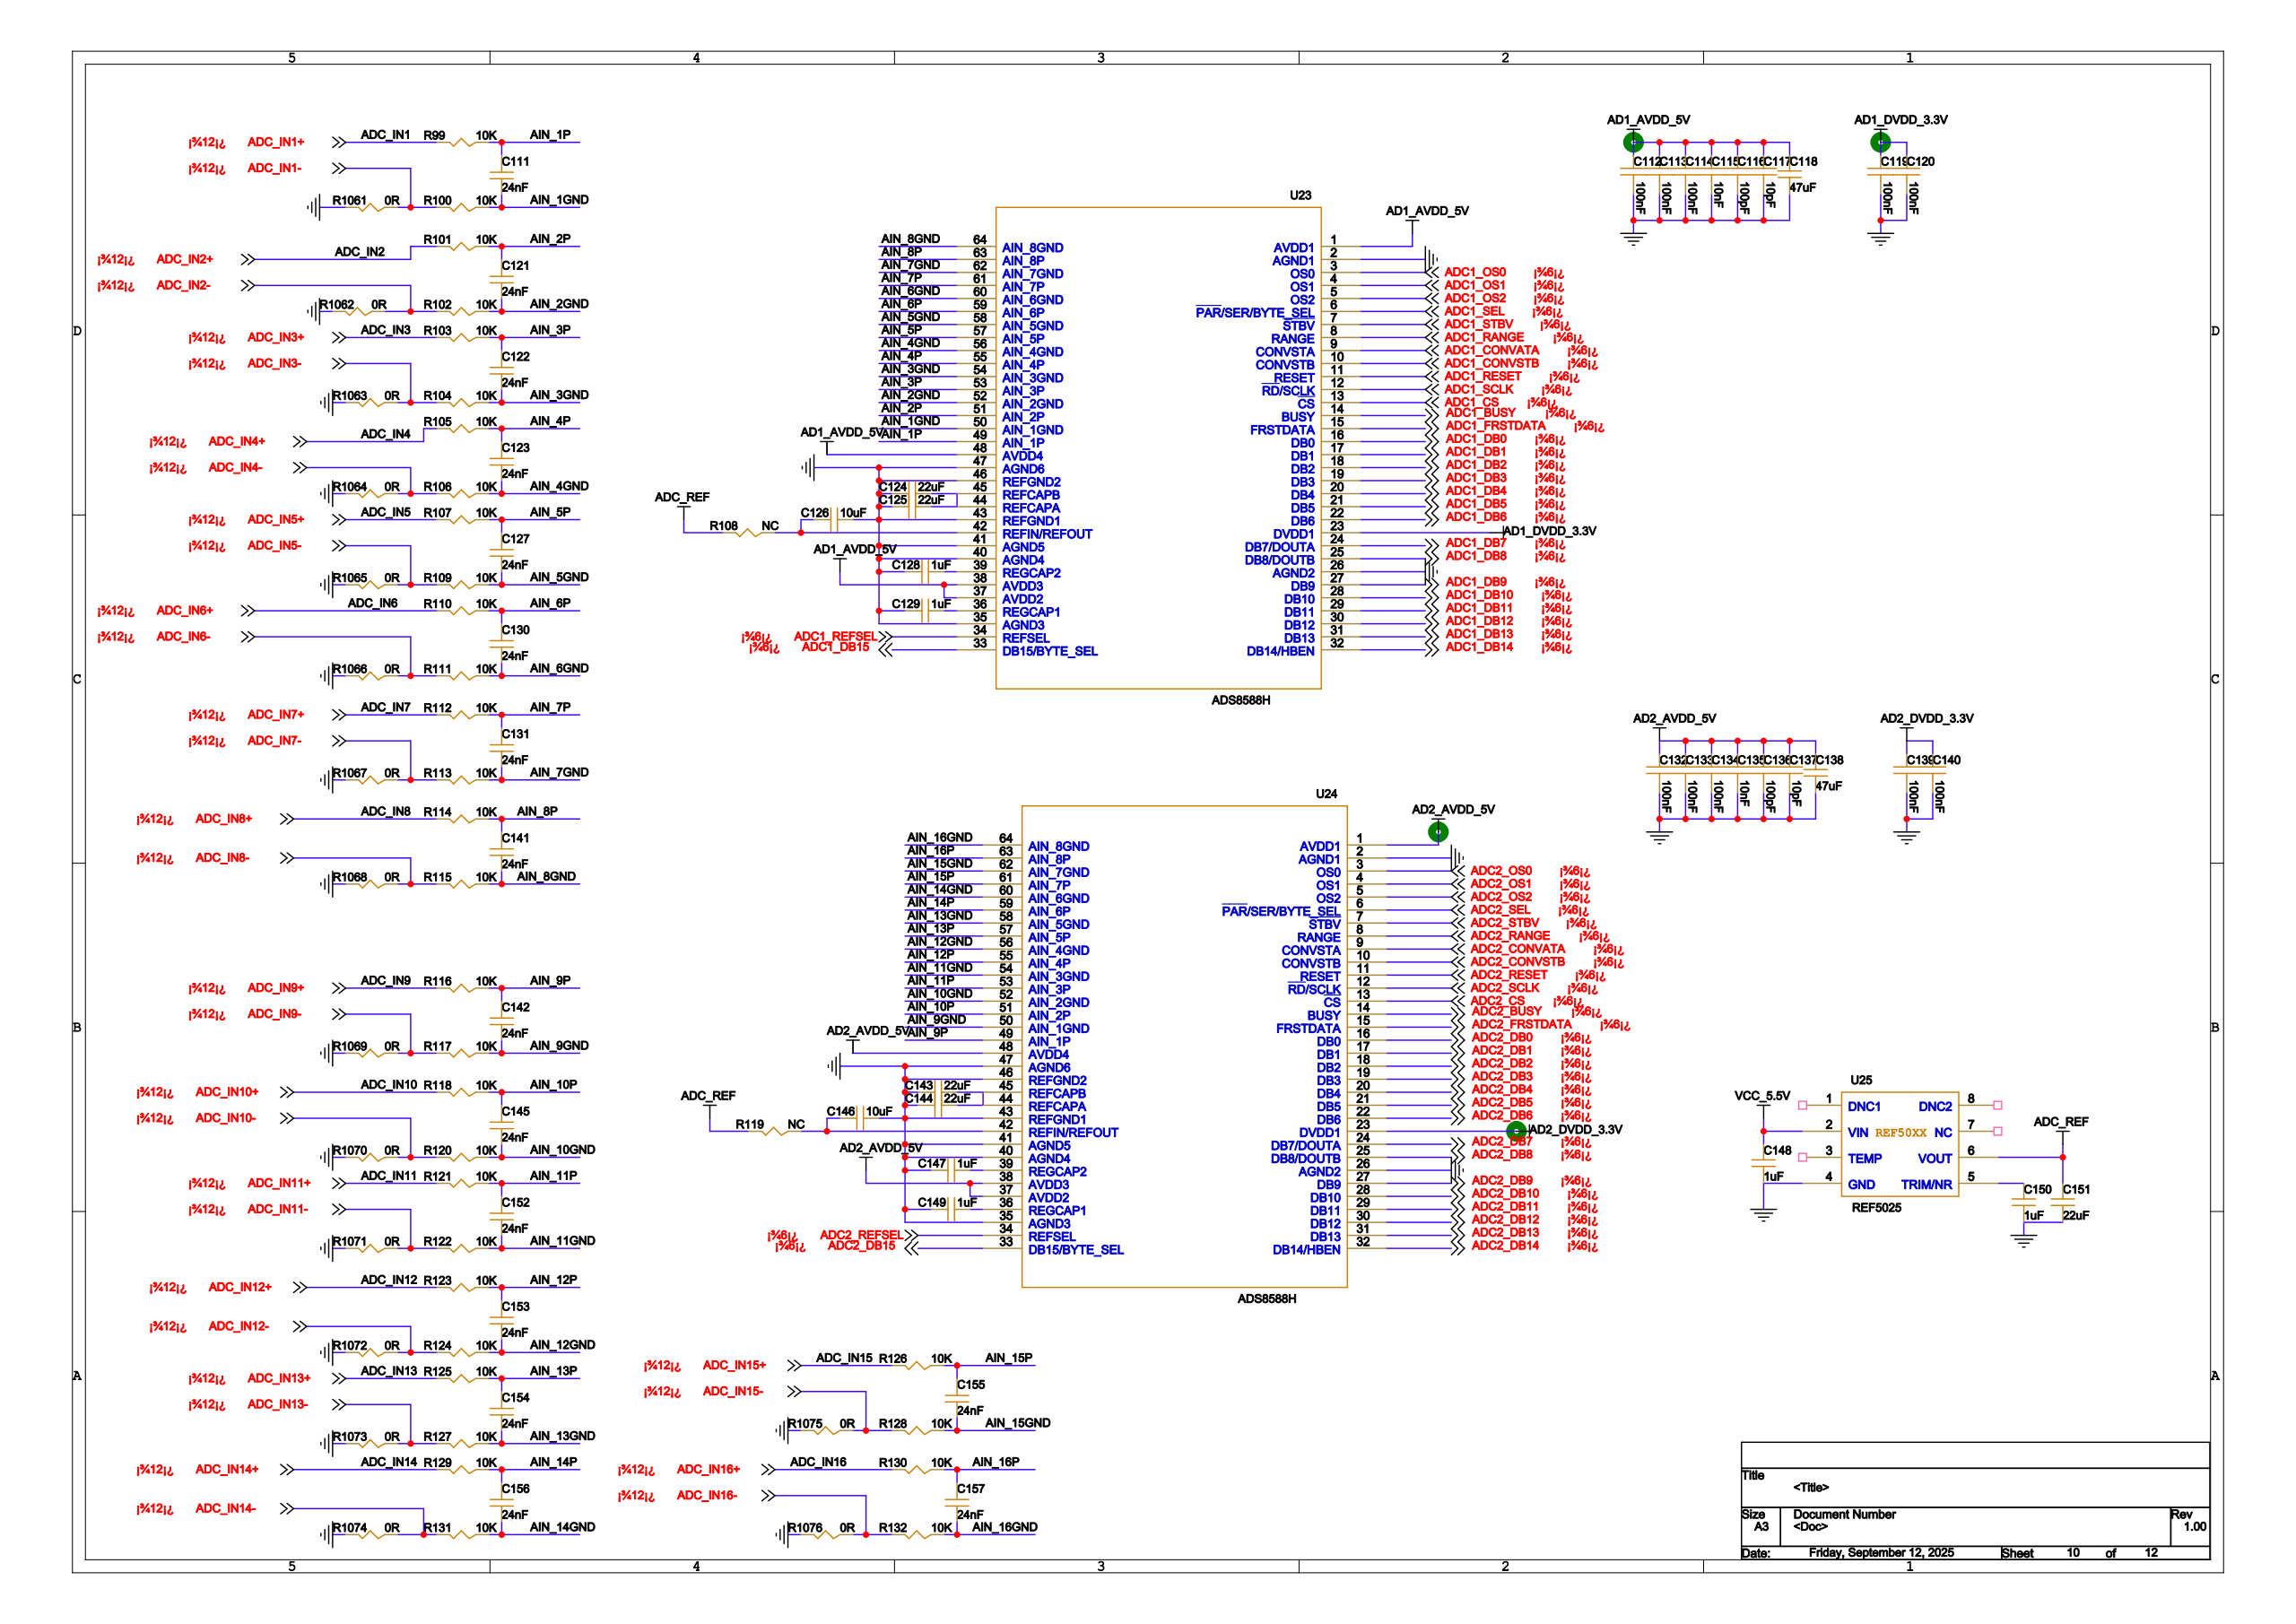Circuit board | Cadence Allegro | 528 parts | 530 nets | one sheet of the schematic
Parts on this sheet (reference | value | footprint):
C111 | 24nF | C0402
C112 | 100nF | C0402
C113 | 100nF | C0402
C114 | 100nF | C0402
C115 | 10nF | C0402
C116 | 100pF | C0402
C117 | 10pF | C0402
C118 | 47uF | C0603
C119 | 100nF | C0402
C120 | 100nF | C0402
C121 | 24nF | C0402
C122 | 24nF | C0402
C123 | 24nF | C0402
C124 | 22uF | C0603
C125 | 22uF | C0603
C126 | 10uF | C0603
C127 | 24nF | C0402
C128 | 1uF | C0402
C129 | 1uF | C0402
C130 | 24nF | C0402
C131 | 24nF | C0402
C132 | 100nF | C0402
C133 | 100nF | C0402
C134 | 100nF | C0402
C135 | 10nF | C0402
C136 | 100pF | C0402
C137 | 10pF | C0402
C138 | 47uF | C0603
C139 | 100nF | C0402
C140 | 100nF | C0402
C141 | 24nF | C0402
C142 | 24nF | C0402
C143 | 22uF | C0603
C144 | 22uF | C0603
C145 | 24nF | C0402
C146 | 10uF | C0603
C147 | 1uF | C0402
C148 | 1uF | C0402
C149 | 1uF | C0402
C150 | 1uF | C0402
C151 | 22uF | C0603
C152 | 24nF | C0402
C153 | 24nF | C0402
C154 | 24nF | C0402
C155 | 24nF | C0402
C156 | 24nF | C0402
C157 | 24nF | C0402
R99 | 10K | R0402
R100 | 10K | R0402
R101 | 10K | R0402
R102 | 10K | R0402
R103 | 10K | R0402
R104 | 10K | R0402
R105 | 10K | R0402
R106 | 10K | R0402
R107 | 10K | R0402
R108 | NC | R0402
R109 | 10K | R0402
R110 | 10K | R0402
R111 | 10K | R0402
R112 | 10K | R0402
R113 | 10K | R0402
R114 | 10K | R0402
R115 | 10K | R0402
R116 | 10K | R0402
R117 | 10K | R0402
R118 | 10K | R0402
R119 | NC | R0402
R120 | 10K | R0402
R121 | 10K | R0402
R122 | 10K | R0402
R123 | 10K | R0402
R124 | 10K | R0402
R125 | 10K | R0402
R126 | 10K | R0402
R127 | 10K | R0402
R128 | 10K | R0402
R129 | 10K | R0402
R130 | 10K | R0402
R131 | 10K | R0402
R132 | 10K | R0402
R1061 | 0R | R0402
R1062 | 0R | R0402
R1063 | 0R | R0402
R1064 | 0R | R0402
R1065 | 0R | R0402
R1066 | 0R | R0402
R1067 | 0R | R0402
R1068 | 0R | R0402
R1069 | 0R | R0402
R1070 | 0R | R0402
R1071 | 0R | R0402
R1072 | 0R | R0402
R1073 | 0R | R0402
R1074 | 0R | R0402
R1075 | 0R | R0402
R1076 | 0R | R0402
U23 | ADS8588H | ADS8588H_LQFP-64
U24 | ADS8588H | ADS8588H_LQFP-64
U25 | REF5025 | SOIC-8
Nets of these parts (net: part-pin ...):
GND: C112-2 C113-2 C114-2 C115-2 C116-2 C117-2 C118-2 C119-2 C120-2 C124-2 C125-2 C126-1 C128-2 C129-2 C132-2 C133-2 C134-2 C135-2 C136-2 C137-2 C138-2 C139-2 C140-2 C143-2 C144-2 C146-1 C147-2 C148-2 C149-2 C150-2 C151-2 R1061-2 R1062-2 R1063-2 R1064-2 R1065-2 R1066-2 R1067-2 R1068-2 R1069-2 R1070-2 R1071-2 R1072-2 R1073-2 R1074-2 R1075-2 R1076-2 U25-4 U23-2 U23-26 U23-35 U23-40 U23-41 U23-43 U23-46 U23-47 U24-2 U24-26 U24-35 U24-40 U24-41 U24-43 U24-46 U24-47
AIN_1GND: C111-1 R100-1 U23-50
AIN_1P: C111-2 R99-1 U23-49
AIN_2GND: C121-1 R102-1 U23-52
AIN_2P: C121-2 R101-1 U23-51
AIN_3GND: C122-1 R104-1 U23-54
AIN_3P: C122-2 R103-1 U23-53
AIN_4GND: C123-1 R106-1 U23-56
AIN_4P: C123-2 R105-1 U23-55
AIN_5GND: C127-1 R109-1 U23-58
AIN_5P: C127-2 R107-1 U23-57
AIN_6GND: C130-1 R111-1 U23-60
AIN_6P: C130-2 R110-1 U23-59
AIN_7GND: C131-1 R113-1 U23-62
AIN_7P: C131-2 R112-1 U23-61
AIN_8GND: C141-1 R115-1 U23-64
AIN_8P: C141-2 R114-1 U23-63
AD1_AVDD_5V: C112-1 C113-1 C114-1 C115-1 C116-1 C117-1 C118-1 U23-1 U23-37 U23-38 U23-48
ADC1_BUSY: U23-14
ADC1_CONVATA: U23-9
ADC1_CONVSTB: U23-10
ADC1_DB0: U23-16
ADC1_DB10: U23-28
ADC1_DB11: U23-29
ADC1_DB12: U23-30
ADC1_DB13: U23-31
ADC1_DB14: U23-32
ADC1_DB15: U23-33
ADC1_DB1: U23-17
ADC1_DB2: U23-18
ADC1_DB3: U23-19
ADC1_DB4: U23-20
ADC1_DB5: U23-21
ADC1_DB6: U23-22
ADC1_DB7: U23-24
ADC1_DB8: U23-25
ADC1_DB9: U23-27
AD1_DVDD_3.3V: C119-1 C120-1 U23-23
ADC1_FRSTDATA: U23-15
ADC1_OS0: U23-3
ADC1_OS1: U23-4
ADC1_OS2: U23-5
ADC1_RANGE: U23-8
N18712329: C124-1 C125-1 U23-44 U23-45
N18712380: C126-2 R108-1 U23-42
ADC1_REFSEL: U23-34
N18712306: C129-1 U23-36
N18712291: C128-1 U23-39
ADC1_RESET: U23-11
ADC1_CS: U23-13
ADC1_SEL: U23-6
ADC1_SCLK: U23-12
ADC1_STBV: U23-7
AIN_9GND: C142-1 R117-1 U24-50
AIN_9P: C142-2 R116-1 U24-49
AIN_10GND: C145-1 R120-1 U24-52
AIN_10P: C145-2 R118-1 U24-51
AIN_11GND: C152-1 R122-1 U24-54
AIN_11P: C152-2 R121-1 U24-53
AIN_12GND: C153-1 R124-1 U24-56
AIN_12P: C153-2 R123-1 U24-55
AIN_13GND: C154-1 R127-1 U24-58
AIN_13P: C154-2 R125-1 U24-57
AIN_14GND: C156-1 R131-1 U24-60
AIN_14P: C156-2 R129-1 U24-59
AIN_15GND: C155-1 R128-1 U24-62
AIN_15P: C155-2 R126-1 U24-61
AIN_16GND: C157-1 R132-1 U24-64
AIN_16P: C157-2 R130-1 U24-63
AD2_AVDD_5V: C132-1 C133-1 C134-1 C135-1 C136-1 C137-1 C138-1 U24-1 U24-37 U24-38 U24-48
ADC2_BUSY: U24-14
ADC2_CONVATA: U24-9
ADC2_CONVSTB: U24-10
ADC2_DB0: U24-16
ADC2_DB10: U24-28
ADC2_DB11: U24-29
ADC2_DB12: U24-30
ADC2_DB13: U24-31
ADC2_DB14: U24-32
ADC2_DB15: U24-33
ADC2_DB1: U24-17
ADC2_DB2: U24-18
ADC2_DB3: U24-19
ADC2_DB4: U24-20
ADC2_DB5: U24-21
ADC2_DB6: U24-22
ADC2_DB7: U24-24
ADC2_DB8: U24-25
ADC2_DB9: U24-27
AD2_DVDD_3.3V: C139-1 C140-1 U24-23
ADC2_FRSTDATA: U24-15
ADC2_OS0: U24-3
ADC2_OS1: U24-4
ADC2_OS2: U24-5
ADC2_RANGE: U24-8
N18717934: C143-1 C144-1 U24-44 U24-45
N18717978: C146-2 R119-1 U24-42
ADC2_REFSEL: U24-34
N18718067: C149-1 U24-36
N18718024: C147-1 U24-39
ADC2_RESET: U24-11
ADC2_CS: U24-13
ADC2_SEL: U24-6
ADC2_SCLK: U24-12
ADC2_STBV: U24-7
ADC_IN10+: R118-2
ADC_IN10-: R120-2 R1070-1
ADC_IN8+: R114-2
ADC_IN8-: R115-2 R1068-1
ADC_IN6+: R110-2
ADC_IN6-: R111-2 R1066-1
ADC_IN16+: R130-2
ADC_IN4+: R105-2
ADC_IN4-: R106-2 R1064-1
ADC_IN2+: R101-2
ADC_IN2-: R102-2 R1062-1
ADC_IN15+: R126-2
ADC_IN15-: R128-2 R1075-1
ADC_IN16-: R132-2 R1076-1
ADC_IN13+: R125-2
ADC_IN13-: R127-2 R1073-1
ADC_IN11+: R121-2
ADC_IN11-: R122-2 R1071-1
ADC_IN9+: R116-2
ADC_IN9-: R117-2 R1069-1
ADC_IN7+: R112-2
ADC_IN7-: R113-2 R1067-1
ADC_IN5+: R107-2
ADC_IN5-: R109-2 R1065-1
ADC_IN3+: R103-2
ADC_IN3-: R104-2 R1063-1
ADC_IN1+: R99-2
ADC_IN1-: R100-2 R1061-1
ADC_IN14+: R129-2
ADC_IN14-: R131-2 R1074-1
ADC_IN12+: R123-2
ADC_IN12-: R124-2 R1072-1
VCC_5.5V: C148-1 U25-2
ADC_REF: C151-1 R108-2 R119-2 U25-6
N18745270: C150-1 U25-5